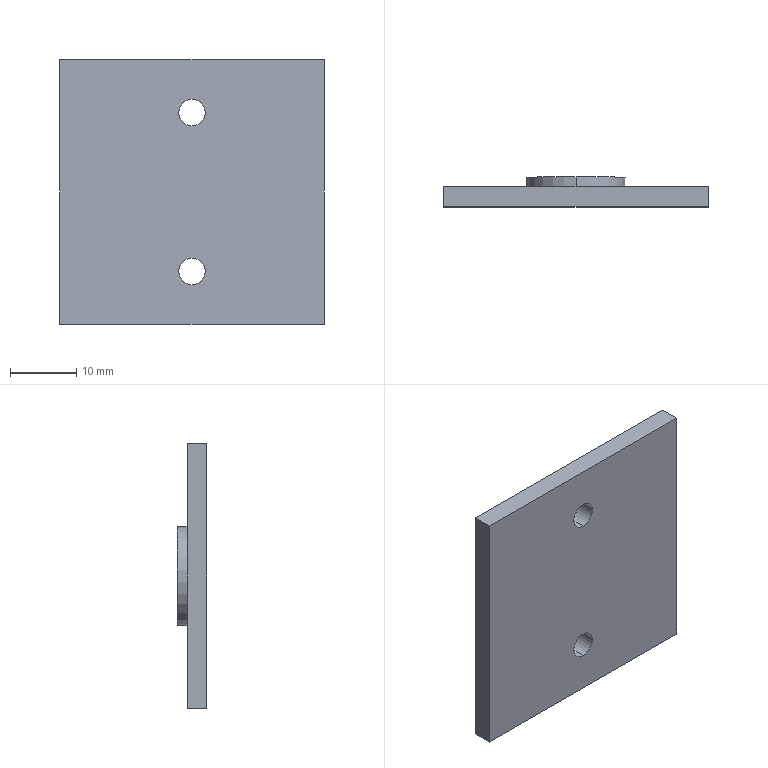Part | STEP file | Guide wheel mechanism revised.sldasm-Part-399 | 1 solid | 13 faces | box 40 x 4.5 x 40 mm | volume 4990 mm3 | plane 7 | cylinder 6 | commonest cylinder face diameters 4 x4 15 x2
STEP:
#1=CARTESIAN_POINT('',(0.,0.,14.));
#2=VERTEX_POINT('',#1);
#3=CARTESIAN_POINT('',(0.,0.,10.));
#4=VERTEX_POINT('',#3);
#5=CARTESIAN_POINT('',(0.,0.,12.));
#6=DIRECTION('',(0.,-1.,0.));
#7=DIRECTION('',(0.,0.,1.));
#8=AXIS2_PLACEMENT_3D('',#5,#6,#7);
#9=CIRCLE('',#8,2.);
#10=EDGE_CURVE('',#2,#4,#9,.T.);
#11=ORIENTED_EDGE('',*,*,#10,.T.);
#12=CARTESIAN_POINT('',(0.,3.,10.));
#13=VERTEX_POINT('',#12);
#14=CARTESIAN_POINT('',(0.,-0.001,10.));
#15=DIRECTION('',(0.,1.,0.));
#16=VECTOR('',#15,1000.);
#17=LINE('',#14,#16);
#18=EDGE_CURVE('',#4,#13,#17,.T.);
#19=ORIENTED_EDGE('',*,*,#18,.T.);
#20=CARTESIAN_POINT('',(0.,3.,14.));
#21=VERTEX_POINT('',#20);
#22=CARTESIAN_POINT('',(0.,3.,12.));
#23=DIRECTION('',(0.,1.,0.));
#24=DIRECTION('',(0.,0.,1.));
#25=AXIS2_PLACEMENT_3D('',#22,#23,#24);
#26=CIRCLE('',#25,2.);
#27=EDGE_CURVE('',#13,#21,#26,.T.);
#28=ORIENTED_EDGE('',*,*,#27,.T.);
#29=CARTESIAN_POINT('',(0.,-0.001,14.));
#30=DIRECTION('',(0.,1.,0.));
#31=VECTOR('',#30,1000.);
#32=LINE('',#29,#31);
#33=EDGE_CURVE('',#2,#21,#32,.T.);
#34=ORIENTED_EDGE('',*,*,#33,.F.);
#35=EDGE_LOOP('',(#11,#19,#28,#34));
#36=FACE_OUTER_BOUND('',#35,.T.);
#37=CARTESIAN_POINT('',(0.,-0.001,12.));
#38=DIRECTION('',(0.,1.,0.));
#39=DIRECTION('',(0.,0.,1.));
#40=AXIS2_PLACEMENT_3D('',#37,#38,#39);
#41=CYLINDRICAL_SURFACE('',#40,2.);
#42=ADVANCED_FACE('',(#36),#41,.F.);
#43=CARTESIAN_POINT('',(0.,0.,-10.));
#44=VERTEX_POINT('',#43);
#45=CARTESIAN_POINT('',(0.,0.,-14.));
#46=VERTEX_POINT('',#45);
#47=CARTESIAN_POINT('',(0.,0.,-12.));
#48=DIRECTION('',(0.,-1.,0.));
#49=DIRECTION('',(0.,0.,1.));
#50=AXIS2_PLACEMENT_3D('',#47,#48,#49);
#51=CIRCLE('',#50,2.);
#52=EDGE_CURVE('',#44,#46,#51,.T.);
#53=ORIENTED_EDGE('',*,*,#52,.T.);
#54=CARTESIAN_POINT('',(0.,3.,-14.));
#55=VERTEX_POINT('',#54);
#56=CARTESIAN_POINT('',(0.,-0.001,-14.));
#57=DIRECTION('',(0.,1.,0.));
#58=VECTOR('',#57,1000.);
#59=LINE('',#56,#58);
#60=EDGE_CURVE('',#46,#55,#59,.T.);
#61=ORIENTED_EDGE('',*,*,#60,.T.);
#62=CARTESIAN_POINT('',(0.,3.,-10.));
#63=VERTEX_POINT('',#62);
#64=CARTESIAN_POINT('',(0.,3.,-12.));
#65=DIRECTION('',(0.,1.,0.));
#66=DIRECTION('',(0.,0.,1.));
#67=AXIS2_PLACEMENT_3D('',#64,#65,#66);
#68=CIRCLE('',#67,2.);
#69=EDGE_CURVE('',#55,#63,#68,.T.);
#70=ORIENTED_EDGE('',*,*,#69,.T.);
#71=CARTESIAN_POINT('',(0.,-0.001,-10.));
#72=DIRECTION('',(0.,1.,0.));
#73=VECTOR('',#72,1000.);
#74=LINE('',#71,#73);
#75=EDGE_CURVE('',#44,#63,#74,.T.);
#76=ORIENTED_EDGE('',*,*,#75,.F.);
#77=EDGE_LOOP('',(#53,#61,#70,#76));
#78=FACE_OUTER_BOUND('',#77,.T.);
#79=CARTESIAN_POINT('',(0.,-0.001,-12.));
#80=DIRECTION('',(0.,1.,0.));
#81=DIRECTION('',(0.,0.,1.));
#82=AXIS2_PLACEMENT_3D('',#79,#80,#81);
#83=CYLINDRICAL_SURFACE('',#82,2.);
#84=ADVANCED_FACE('',(#78),#83,.F.);
#85=CARTESIAN_POINT('',(0.,4.5,7.5));
#86=VERTEX_POINT('',#85);
#87=CARTESIAN_POINT('',(0.,4.5,-7.5));
#88=VERTEX_POINT('',#87);
#89=CARTESIAN_POINT('',(0.,4.5,0.));
#90=DIRECTION('',(0.,1.,0.));
#91=DIRECTION('',(0.,0.,1.));
#92=AXIS2_PLACEMENT_3D('',#89,#90,#91);
#93=CIRCLE('',#92,7.5);
#94=EDGE_CURVE('',#86,#88,#93,.T.);
#95=ORIENTED_EDGE('',*,*,#94,.F.);
#96=CARTESIAN_POINT('',(0.,3.,7.5));
#97=VERTEX_POINT('',#96);
#98=CARTESIAN_POINT('',(0.,4.5,7.5));
#99=DIRECTION('',(0.,-1.,0.));
#100=VECTOR('',#99,1000.);
#101=LINE('',#98,#100);
#102=EDGE_CURVE('',#86,#97,#101,.T.);
#103=ORIENTED_EDGE('',*,*,#102,.T.);
#104=CARTESIAN_POINT('',(0.,3.,-7.5));
#105=VERTEX_POINT('',#104);
#106=CARTESIAN_POINT('',(0.,3.,0.));
#107=DIRECTION('',(0.,1.,0.));
#108=DIRECTION('',(0.,0.,1.));
#109=AXIS2_PLACEMENT_3D('',#106,#107,#108);
#110=CIRCLE('',#109,7.5);
#111=EDGE_CURVE('',#97,#105,#110,.T.);
#112=ORIENTED_EDGE('',*,*,#111,.T.);
#113=CARTESIAN_POINT('',(0.,4.5,-7.5));
#114=DIRECTION('',(0.,-1.,0.));
#115=VECTOR('',#114,1000.);
#116=LINE('',#113,#115);
#117=EDGE_CURVE('',#88,#105,#116,.T.);
#118=ORIENTED_EDGE('',*,*,#117,.F.);
#119=EDGE_LOOP('',(#95,#103,#112,#118));
#120=FACE_OUTER_BOUND('',#119,.T.);
#121=CARTESIAN_POINT('',(0.,4.5,0.));
#122=DIRECTION('',(0.,-1.,0.));
#123=DIRECTION('',(0.,0.,-1.));
#124=AXIS2_PLACEMENT_3D('',#121,#122,#123);
#125=CYLINDRICAL_SURFACE('',#124,7.5);
#126=ADVANCED_FACE('',(#120),#125,.T.);
#127=CARTESIAN_POINT('',(0.,3.,12.));
#128=DIRECTION('',(0.,1.,0.));
#129=DIRECTION('',(0.,0.,1.));
#130=AXIS2_PLACEMENT_3D('',#127,#128,#129);
#131=CIRCLE('',#130,2.);
#132=EDGE_CURVE('',#21,#13,#131,.T.);
#133=ORIENTED_EDGE('',*,*,#132,.F.);
#134=ORIENTED_EDGE('',*,*,#27,.F.);
#135=EDGE_LOOP('',(#133,#134));
#136=FACE_BOUND('',#135,.T.);
#137=CARTESIAN_POINT('',(0.,3.,-12.));
#138=DIRECTION('',(0.,1.,0.));
#139=DIRECTION('',(0.,0.,1.));
#140=AXIS2_PLACEMENT_3D('',#137,#138,#139);
#141=CIRCLE('',#140,2.);
#142=EDGE_CURVE('',#63,#55,#141,.T.);
#143=ORIENTED_EDGE('',*,*,#142,.F.);
#144=ORIENTED_EDGE('',*,*,#69,.F.);
#145=EDGE_LOOP('',(#143,#144));
#146=FACE_BOUND('',#145,.T.);
#147=CARTESIAN_POINT('',(20.,3.,20.));
#148=VERTEX_POINT('',#147);
#149=CARTESIAN_POINT('',(20.,3.,-20.));
#150=VERTEX_POINT('',#149);
#151=CARTESIAN_POINT('',(20.,3.,20.));
#152=DIRECTION('',(0.,0.,-1.));
#153=VECTOR('',#152,1000.);
#154=LINE('',#151,#153);
#155=EDGE_CURVE('',#148,#150,#154,.T.);
#156=ORIENTED_EDGE('',*,*,#155,.T.);
#157=CARTESIAN_POINT('',(-20.,3.,-20.));
#158=VERTEX_POINT('',#157);
#159=CARTESIAN_POINT('',(20.,3.,-20.));
#160=DIRECTION('',(-1.,0.,0.));
#161=VECTOR('',#160,1000.);
#162=LINE('',#159,#161);
#163=EDGE_CURVE('',#150,#158,#162,.T.);
#164=ORIENTED_EDGE('',*,*,#163,.T.);
#165=CARTESIAN_POINT('',(-20.,3.,20.));
#166=VERTEX_POINT('',#165);
#167=CARTESIAN_POINT('',(-20.,3.,20.));
#168=DIRECTION('',(0.,0.,-1.));
#169=VECTOR('',#168,1000.);
#170=LINE('',#167,#169);
#171=EDGE_CURVE('',#166,#158,#170,.T.);
#172=ORIENTED_EDGE('',*,*,#171,.F.);
#173=CARTESIAN_POINT('',(20.,3.,20.));
#174=DIRECTION('',(-1.,0.,0.));
#175=VECTOR('',#174,1000.);
#176=LINE('',#173,#175);
#177=EDGE_CURVE('',#148,#166,#176,.T.);
#178=ORIENTED_EDGE('',*,*,#177,.F.);
#179=EDGE_LOOP('',(#156,#164,#172,#178));
#180=FACE_OUTER_BOUND('',#179,.T.);
#181=CARTESIAN_POINT('',(0.,3.,0.));
#182=DIRECTION('',(0.,1.,0.));
#183=DIRECTION('',(0.,0.,1.));
#184=AXIS2_PLACEMENT_3D('',#181,#182,#183);
#185=CIRCLE('',#184,7.5);
#186=EDGE_CURVE('',#105,#97,#185,.T.);
#187=ORIENTED_EDGE('',*,*,#186,.F.);
#188=ORIENTED_EDGE('',*,*,#111,.F.);
#189=EDGE_LOOP('',(#187,#188));
#190=FACE_BOUND('',#189,.T.);
#191=CARTESIAN_POINT('',(0.,3.,0.));
#192=DIRECTION('',(0.,1.,0.));
#193=DIRECTION('',(0.,0.,1.));
#194=AXIS2_PLACEMENT_3D('',#191,#192,#193);
#195=PLANE('',#194);
#196=ADVANCED_FACE('',(#136,#146,#180,#190),#195,.T.);
#197=CARTESIAN_POINT('',(20.,0.,20.));
#198=VERTEX_POINT('',#197);
#199=CARTESIAN_POINT('',(20.,0.,-20.));
#200=VERTEX_POINT('',#199);
#201=CARTESIAN_POINT('',(20.,0.,20.));
#202=DIRECTION('',(0.,0.,-1.));
#203=VECTOR('',#202,1000.);
#204=LINE('',#201,#203);
#205=EDGE_CURVE('',#198,#200,#204,.T.);
#206=ORIENTED_EDGE('',*,*,#205,.T.);
#207=CARTESIAN_POINT('',(20.,3.,-20.));
#208=DIRECTION('',(0.,-1.,0.));
#209=VECTOR('',#208,1000.);
#210=LINE('',#207,#209);
#211=EDGE_CURVE('',#150,#200,#210,.T.);
#212=ORIENTED_EDGE('',*,*,#211,.F.);
#213=ORIENTED_EDGE('',*,*,#155,.F.);
#214=CARTESIAN_POINT('',(20.,3.,20.));
#215=DIRECTION('',(0.,-1.,0.));
#216=VECTOR('',#215,1000.);
#217=LINE('',#214,#216);
#218=EDGE_CURVE('',#148,#198,#217,.T.);
#219=ORIENTED_EDGE('',*,*,#218,.T.);
#220=EDGE_LOOP('',(#206,#212,#213,#219));
#221=FACE_OUTER_BOUND('',#220,.T.);
#222=CARTESIAN_POINT('',(20.,3.,20.));
#223=DIRECTION('',(-1.,0.,0.));
#224=DIRECTION('',(0.,0.,1.));
#225=AXIS2_PLACEMENT_3D('',#222,#223,#224);
#226=PLANE('',#225);
#227=ADVANCED_FACE('',(#221),#226,.F.);
#228=CARTESIAN_POINT('',(-20.,0.,-20.));
#229=VERTEX_POINT('',#228);
#230=CARTESIAN_POINT('',(20.,0.,-20.));
#231=DIRECTION('',(-1.,0.,0.));
#232=VECTOR('',#231,1000.);
#233=LINE('',#230,#232);
#234=EDGE_CURVE('',#200,#229,#233,.T.);
#235=ORIENTED_EDGE('',*,*,#234,.T.);
#236=CARTESIAN_POINT('',(-20.,3.,-20.));
#237=DIRECTION('',(0.,-1.,0.));
#238=VECTOR('',#237,1000.);
#239=LINE('',#236,#238);
#240=EDGE_CURVE('',#158,#229,#239,.T.);
#241=ORIENTED_EDGE('',*,*,#240,.F.);
#242=ORIENTED_EDGE('',*,*,#163,.F.);
#243=ORIENTED_EDGE('',*,*,#211,.T.);
#244=EDGE_LOOP('',(#235,#241,#242,#243));
#245=FACE_OUTER_BOUND('',#244,.T.);
#246=CARTESIAN_POINT('',(20.,3.,-20.));
#247=DIRECTION('',(0.,0.,1.));
#248=DIRECTION('',(1.,0.,0.));
#249=AXIS2_PLACEMENT_3D('',#246,#247,#248);
#250=PLANE('',#249);
#251=ADVANCED_FACE('',(#245),#250,.F.);
#252=CARTESIAN_POINT('',(-20.,0.,20.));
#253=VERTEX_POINT('',#252);
#254=CARTESIAN_POINT('',(-20.,0.,20.));
#255=DIRECTION('',(0.,0.,-1.));
#256=VECTOR('',#255,1000.);
#257=LINE('',#254,#256);
#258=EDGE_CURVE('',#253,#229,#257,.T.);
#259=ORIENTED_EDGE('',*,*,#258,.F.);
#260=CARTESIAN_POINT('',(-20.,3.,20.));
#261=DIRECTION('',(0.,-1.,0.));
#262=VECTOR('',#261,1000.);
#263=LINE('',#260,#262);
#264=EDGE_CURVE('',#166,#253,#263,.T.);
#265=ORIENTED_EDGE('',*,*,#264,.F.);
#266=ORIENTED_EDGE('',*,*,#171,.T.);
#267=ORIENTED_EDGE('',*,*,#240,.T.);
#268=EDGE_LOOP('',(#259,#265,#266,#267));
#269=FACE_OUTER_BOUND('',#268,.T.);
#270=CARTESIAN_POINT('',(-20.,3.,20.));
#271=DIRECTION('',(-1.,0.,0.));
#272=DIRECTION('',(0.,0.,1.));
#273=AXIS2_PLACEMENT_3D('',#270,#271,#272);
#274=PLANE('',#273);
#275=ADVANCED_FACE('',(#269),#274,.T.);
#276=CARTESIAN_POINT('',(20.,0.,20.));
#277=DIRECTION('',(-1.,0.,0.));
#278=VECTOR('',#277,1000.);
#279=LINE('',#276,#278);
#280=EDGE_CURVE('',#198,#253,#279,.T.);
#281=ORIENTED_EDGE('',*,*,#280,.F.);
#282=ORIENTED_EDGE('',*,*,#218,.F.);
#283=ORIENTED_EDGE('',*,*,#177,.T.);
#284=ORIENTED_EDGE('',*,*,#264,.T.);
#285=EDGE_LOOP('',(#281,#282,#283,#284));
#286=FACE_OUTER_BOUND('',#285,.T.);
#287=CARTESIAN_POINT('',(20.,3.,20.));
#288=DIRECTION('',(0.,0.,1.));
#289=DIRECTION('',(1.,0.,0.));
#290=AXIS2_PLACEMENT_3D('',#287,#288,#289);
#291=PLANE('',#290);
#292=ADVANCED_FACE('',(#286),#291,.T.);
#293=ORIENTED_EDGE('',*,*,#10,.F.);
#294=CARTESIAN_POINT('',(0.,0.,12.));
#295=DIRECTION('',(0.,-1.,0.));
#296=DIRECTION('',(0.,0.,1.));
#297=AXIS2_PLACEMENT_3D('',#294,#295,#296);
#298=CIRCLE('',#297,2.);
#299=EDGE_CURVE('',#4,#2,#298,.T.);
#300=ORIENTED_EDGE('',*,*,#299,.F.);
#301=EDGE_LOOP('',(#293,#300));
#302=FACE_BOUND('',#301,.T.);
#303=ORIENTED_EDGE('',*,*,#52,.F.);
#304=CARTESIAN_POINT('',(0.,0.,-12.));
#305=DIRECTION('',(0.,-1.,0.));
#306=DIRECTION('',(0.,0.,1.));
#307=AXIS2_PLACEMENT_3D('',#304,#305,#306);
#308=CIRCLE('',#307,2.);
#309=EDGE_CURVE('',#46,#44,#308,.T.);
#310=ORIENTED_EDGE('',*,*,#309,.F.);
#311=EDGE_LOOP('',(#303,#310));
#312=FACE_BOUND('',#311,.T.);
#313=ORIENTED_EDGE('',*,*,#205,.F.);
#314=ORIENTED_EDGE('',*,*,#280,.T.);
#315=ORIENTED_EDGE('',*,*,#258,.T.);
#316=ORIENTED_EDGE('',*,*,#234,.F.);
#317=EDGE_LOOP('',(#313,#314,#315,#316));
#318=FACE_OUTER_BOUND('',#317,.T.);
#319=CARTESIAN_POINT('',(0.,0.,0.));
#320=DIRECTION('',(0.,1.,0.));
#321=DIRECTION('',(0.,0.,1.));
#322=AXIS2_PLACEMENT_3D('',#319,#320,#321);
#323=PLANE('',#322);
#324=ADVANCED_FACE('',(#302,#312,#318),#323,.F.);
#325=ORIENTED_EDGE('',*,*,#102,.F.);
#326=CARTESIAN_POINT('',(0.,4.5,0.));
#327=DIRECTION('',(0.,1.,0.));
#328=DIRECTION('',(0.,0.,1.));
#329=AXIS2_PLACEMENT_3D('',#326,#327,#328);
#330=CIRCLE('',#329,7.5);
#331=EDGE_CURVE('',#88,#86,#330,.T.);
#332=ORIENTED_EDGE('',*,*,#331,.F.);
#333=ORIENTED_EDGE('',*,*,#117,.T.);
#334=ORIENTED_EDGE('',*,*,#186,.T.);
#335=EDGE_LOOP('',(#325,#332,#333,#334));
#336=FACE_OUTER_BOUND('',#335,.T.);
#337=CARTESIAN_POINT('',(0.,4.5,0.));
#338=DIRECTION('',(0.,-1.,0.));
#339=DIRECTION('',(0.,0.,-1.));
#340=AXIS2_PLACEMENT_3D('',#337,#338,#339);
#341=CYLINDRICAL_SURFACE('',#340,7.5);
#342=ADVANCED_FACE('',(#336),#341,.T.);
#343=ORIENTED_EDGE('',*,*,#331,.T.);
#344=ORIENTED_EDGE('',*,*,#94,.T.);
#345=EDGE_LOOP('',(#343,#344));
#346=FACE_OUTER_BOUND('',#345,.T.);
#347=CARTESIAN_POINT('',(0.,4.5,0.));
#348=DIRECTION('',(0.,1.,0.));
#349=DIRECTION('',(0.,0.,1.));
#350=AXIS2_PLACEMENT_3D('',#347,#348,#349);
#351=PLANE('',#350);
#352=ADVANCED_FACE('',(#346),#351,.T.);
#353=ORIENTED_EDGE('',*,*,#60,.F.);
#354=ORIENTED_EDGE('',*,*,#309,.T.);
#355=ORIENTED_EDGE('',*,*,#75,.T.);
#356=ORIENTED_EDGE('',*,*,#142,.T.);
#357=EDGE_LOOP('',(#353,#354,#355,#356));
#358=FACE_OUTER_BOUND('',#357,.T.);
#359=CARTESIAN_POINT('',(0.,-0.001,-12.));
#360=DIRECTION('',(0.,1.,0.));
#361=DIRECTION('',(0.,0.,1.));
#362=AXIS2_PLACEMENT_3D('',#359,#360,#361);
#363=CYLINDRICAL_SURFACE('',#362,2.);
#364=ADVANCED_FACE('',(#358),#363,.F.);
#365=ORIENTED_EDGE('',*,*,#18,.F.);
#366=ORIENTED_EDGE('',*,*,#299,.T.);
#367=ORIENTED_EDGE('',*,*,#33,.T.);
#368=ORIENTED_EDGE('',*,*,#132,.T.);
#369=EDGE_LOOP('',(#365,#366,#367,#368));
#370=FACE_OUTER_BOUND('',#369,.T.);
#371=CARTESIAN_POINT('',(0.,-0.001,12.));
#372=DIRECTION('',(0.,1.,0.));
#373=DIRECTION('',(0.,0.,1.));
#374=AXIS2_PLACEMENT_3D('',#371,#372,#373);
#375=CYLINDRICAL_SURFACE('',#374,2.);
#376=ADVANCED_FACE('',(#370),#375,.F.);
#377=CLOSED_SHELL('',(#42,#84,#126,#196,#227,#251,#275,#292,#324,#342,#352,#364,#376));
#378=MANIFOLD_SOLID_BREP('',#377);
#379=CARTESIAN_POINT('',(0.,0.,0.));
#380=DIRECTION('',(0.,0.,1.));
#381=DIRECTION('',(1.,0.,0.));
#382=AXIS2_PLACEMENT_3D('',#379,#380,#381);
#383=(LENGTH_UNIT()NAMED_UNIT(*)SI_UNIT(.MILLI.,.METRE.));
#384=UNCERTAINTY_MEASURE_WITH_UNIT(LENGTH_MEASURE(0.00001),#383,'','');
#385=(NAMED_UNIT(*)PLANE_ANGLE_UNIT()SI_UNIT($,.RADIAN.));
#386=(NAMED_UNIT(*)SI_UNIT($,.STERADIAN.)SOLID_ANGLE_UNIT());
#387=(GEOMETRIC_REPRESENTATION_CONTEXT(3)GLOBAL_UNCERTAINTY_ASSIGNED_CONTEXT((#384))GLOBAL_UNIT_ASSIGNED_CONTEXT((#383,#385,#386))REPRESENTATION_CONTEXT('',''));
#388=ADVANCED_BREP_SHAPE_REPRESENTATION('',(#378,#382),#387);